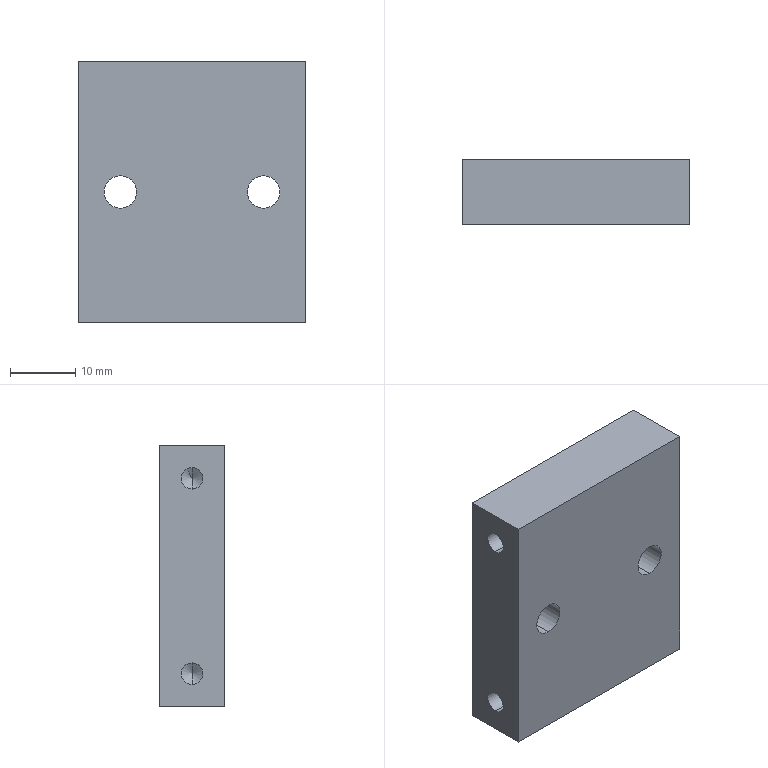Part | STEP file | 0243_215_Plate | 1 solid | 26 faces | box 35 x 10 x 40 mm | volume 13250 mm3 | cylinder 12 | cone 8 | plane 6 | commonest cylinder face diameters 3.3 x8 5 x4